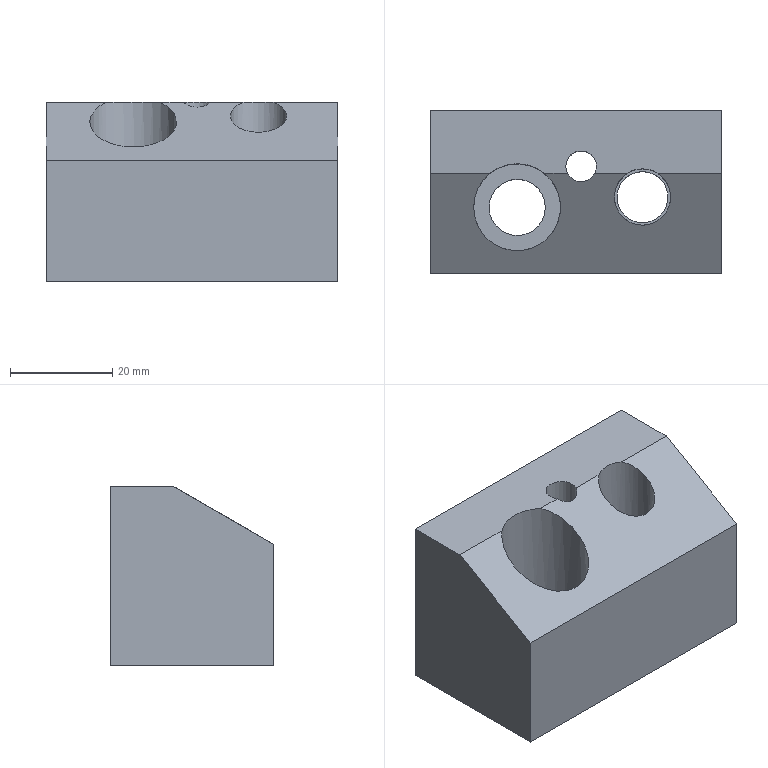Part | STEP file | lll_id4166_x_t | 1 solid | 14 faces | box 57 x 32 x 35 mm | volume 48436 mm3 | plane 9 | cylinder 5 | commonest cylinder face diameters 11 x2 6 x1 10 x1 17 x1
STEP:
#1=CARTESIAN_POINT('',(3855.,-59.75,-35.));
#2=VERTEX_POINT('',#1);
#3=CARTESIAN_POINT('',(3849.5,-59.75,-35.));
#4=DIRECTION('',(0.,0.,1.));
#5=DIRECTION('',(1.,0.,0.));
#6=AXIS2_PLACEMENT_3D('',#3,#4,#5);
#7=CIRCLE('',#6,5.5);
#8=EDGE_CURVE('',#2,#2,#7,.T.);
#9=ORIENTED_EDGE('',*,*,#8,.T.);
#10=EDGE_LOOP('',(#9));
#11=FACE_BOUND('',#10,.T.);
#12=CARTESIAN_POINT('',(3832.5,-40.75,-35.));
#13=VERTEX_POINT('',#12);
#14=CARTESIAN_POINT('',(3832.5,-72.75,-35.));
#15=VERTEX_POINT('',#14);
#16=CARTESIAN_POINT('',(3832.5,-36.5,-35.));
#17=DIRECTION('',(0.,-1.,0.));
#18=VECTOR('',#17,1.);
#19=LINE('',#16,#18);
#20=EDGE_CURVE('',#13,#15,#19,.T.);
#21=ORIENTED_EDGE('',*,*,#20,.F.);
#22=CARTESIAN_POINT('',(3889.5,-40.75,-35.));
#23=VERTEX_POINT('',#22);
#24=CARTESIAN_POINT('',(3854.,-40.75,-35.));
#25=DIRECTION('',(-1.,0.,0.));
#26=VECTOR('',#25,1.);
#27=LINE('',#24,#26);
#28=EDGE_CURVE('',#23,#13,#27,.T.);
#29=ORIENTED_EDGE('',*,*,#28,.F.);
#30=CARTESIAN_POINT('',(3889.5,-72.75,-35.));
#31=VERTEX_POINT('',#30);
#32=CARTESIAN_POINT('',(3889.5,-36.5,-35.));
#33=DIRECTION('',(0.,1.,0.));
#34=VECTOR('',#33,1.);
#35=LINE('',#32,#34);
#36=EDGE_CURVE('',#31,#23,#35,.T.);
#37=ORIENTED_EDGE('',*,*,#36,.F.);
#38=CARTESIAN_POINT('',(3854.,-72.75,-35.));
#39=DIRECTION('',(1.,0.,0.));
#40=VECTOR('',#39,1.);
#41=LINE('',#38,#40);
#42=EDGE_CURVE('',#15,#31,#41,.T.);
#43=ORIENTED_EDGE('',*,*,#42,.F.);
#44=EDGE_LOOP('',(#21,#29,#37,#43));
#45=FACE_BOUND('',#44,.T.);
#46=CARTESIAN_POINT('',(3874.,-62.75,-35.));
#47=VERTEX_POINT('',#46);
#48=CARTESIAN_POINT('',(3874.,-57.75,-35.));
#49=DIRECTION('',(0.,0.,1.));
#50=DIRECTION('',(0.,-1.,0.));
#51=AXIS2_PLACEMENT_3D('',#48,#49,#50);
#52=CIRCLE('',#51,5.);
#53=EDGE_CURVE('',#47,#47,#52,.T.);
#54=ORIENTED_EDGE('',*,*,#53,.T.);
#55=EDGE_LOOP('',(#54));
#56=FACE_BOUND('',#55,.T.);
#57=CARTESIAN_POINT('',(3859.,-51.75,-35.));
#58=VERTEX_POINT('',#57);
#59=CARTESIAN_POINT('',(3862.,-51.75,-35.));
#60=DIRECTION('',(0.,0.,-1.));
#61=DIRECTION('',(-1.,0.,0.));
#62=AXIS2_PLACEMENT_3D('',#59,#60,#61);
#63=CIRCLE('',#62,3.);
#64=EDGE_CURVE('',#58,#58,#63,.T.);
#65=ORIENTED_EDGE('',*,*,#64,.F.);
#66=EDGE_LOOP('',(#65));
#67=FACE_BOUND('',#66,.T.);
#68=CARTESIAN_POINT('',(3854.,-36.5,-35.));
#69=DIRECTION('',(0.,0.,-1.));
#70=DIRECTION('',(0.,-1.,0.));
#71=AXIS2_PLACEMENT_3D('',#68,#69,#70);
#72=PLANE('',#71);
#73=ADVANCED_FACE('',(#11,#45,#56,#67),#72,.T.);
#74=CARTESIAN_POINT('',(3870.966,-53.163,0.));
#75=VERTEX_POINT('',#74);
#76=CARTESIAN_POINT('',(3864.647,-53.163,0.));
#77=VERTEX_POINT('',#76);
#78=CARTESIAN_POINT('',(3854.,-53.163,0.));
#79=DIRECTION('',(-1.,0.,0.));
#80=VECTOR('',#79,1.);
#81=LINE('',#78,#80);
#82=EDGE_CURVE('',#75,#77,#81,.T.);
#83=ORIENTED_EDGE('',*,*,#82,.F.);
#84=CARTESIAN_POINT('',(3877.034,-53.163,0.));
#85=VERTEX_POINT('',#84);
#86=CARTESIAN_POINT('',(3874.,-57.75,0.));
#87=DIRECTION('',(0.,0.,1.));
#88=DIRECTION('',(0.,1.,0.));
#89=AXIS2_PLACEMENT_3D('',#86,#87,#88);
#90=CIRCLE('',#89,5.5);
#91=EDGE_CURVE('',#85,#75,#90,.T.);
#92=ORIENTED_EDGE('',*,*,#91,.F.);
#93=CARTESIAN_POINT('',(3889.5,-53.163,0.));
#94=VERTEX_POINT('',#93);
#95=CARTESIAN_POINT('',(3854.,-53.163,0.));
#96=DIRECTION('',(-1.,0.,0.));
#97=VECTOR('',#96,1.);
#98=LINE('',#95,#97);
#99=EDGE_CURVE('',#94,#85,#98,.T.);
#100=ORIENTED_EDGE('',*,*,#99,.F.);
#101=CARTESIAN_POINT('',(3889.5,-40.75,0.));
#102=VERTEX_POINT('',#101);
#103=CARTESIAN_POINT('',(3889.5,-36.5,0.));
#104=DIRECTION('',(0.,-1.,0.));
#105=VECTOR('',#104,1.);
#106=LINE('',#103,#105);
#107=EDGE_CURVE('',#102,#94,#106,.T.);
#108=ORIENTED_EDGE('',*,*,#107,.F.);
#109=CARTESIAN_POINT('',(3832.5,-40.75,0.));
#110=VERTEX_POINT('',#109);
#111=CARTESIAN_POINT('',(3854.,-40.75,0.));
#112=DIRECTION('',(1.,0.,0.));
#113=VECTOR('',#112,1.);
#114=LINE('',#111,#113);
#115=EDGE_CURVE('',#110,#102,#114,.T.);
#116=ORIENTED_EDGE('',*,*,#115,.F.);
#117=CARTESIAN_POINT('',(3832.5,-53.163,0.));
#118=VERTEX_POINT('',#117);
#119=CARTESIAN_POINT('',(3832.5,-36.5,0.));
#120=DIRECTION('',(0.,1.,0.));
#121=VECTOR('',#120,1.);
#122=LINE('',#119,#121);
#123=EDGE_CURVE('',#118,#110,#122,.T.);
#124=ORIENTED_EDGE('',*,*,#123,.F.);
#125=CARTESIAN_POINT('',(3844.128,-53.163,0.));
#126=VERTEX_POINT('',#125);
#127=CARTESIAN_POINT('',(3854.,-53.163,0.));
#128=DIRECTION('',(-1.,0.,0.));
#129=VECTOR('',#128,1.);
#130=LINE('',#127,#129);
#131=EDGE_CURVE('',#126,#118,#130,.T.);
#132=ORIENTED_EDGE('',*,*,#131,.F.);
#133=CARTESIAN_POINT('',(3854.872,-53.163,0.));
#134=VERTEX_POINT('',#133);
#135=CARTESIAN_POINT('',(3849.5,-59.75,0.));
#136=DIRECTION('',(0.,0.,1.));
#137=DIRECTION('',(-1.,0.,0.));
#138=AXIS2_PLACEMENT_3D('',#135,#136,#137);
#139=CIRCLE('',#138,8.5);
#140=EDGE_CURVE('',#134,#126,#139,.T.);
#141=ORIENTED_EDGE('',*,*,#140,.F.);
#142=CARTESIAN_POINT('',(3859.354,-53.163,0.));
#143=VERTEX_POINT('',#142);
#144=CARTESIAN_POINT('',(3854.,-53.163,0.));
#145=DIRECTION('',(-1.,0.,0.));
#146=VECTOR('',#145,1.);
#147=LINE('',#144,#146);
#148=EDGE_CURVE('',#143,#134,#147,.T.);
#149=ORIENTED_EDGE('',*,*,#148,.F.);
#150=CARTESIAN_POINT('',(3862.,-51.75,0.));
#151=DIRECTION('',(0.,0.,1.));
#152=DIRECTION('',(1.,0.,0.));
#153=AXIS2_PLACEMENT_3D('',#150,#151,#152);
#154=CIRCLE('',#153,3.);
#155=EDGE_CURVE('',#77,#143,#154,.T.);
#156=ORIENTED_EDGE('',*,*,#155,.F.);
#157=EDGE_LOOP('',(#83,#92,#100,#108,#116,#124,#132,#141,#149,#156));
#158=FACE_OUTER_BOUND('',#157,.T.);
#159=CARTESIAN_POINT('',(3854.,-36.5,0.));
#160=DIRECTION('',(0.,0.,1.));
#161=DIRECTION('',(0.,1.,0.));
#162=AXIS2_PLACEMENT_3D('',#159,#160,#161);
#163=PLANE('',#162);
#164=ADVANCED_FACE('',(#158),#163,.T.);
#165=CARTESIAN_POINT('',(3844.,-59.75,-22.));
#166=VERTEX_POINT('',#165);
#167=CARTESIAN_POINT('',(3849.5,-59.75,-22.));
#168=DIRECTION('',(0.,0.,-1.));
#169=DIRECTION('',(-1.,0.,0.));
#170=AXIS2_PLACEMENT_3D('',#167,#168,#169);
#171=CIRCLE('',#170,5.5);
#172=EDGE_CURVE('',#166,#166,#171,.T.);
#173=ORIENTED_EDGE('',*,*,#172,.F.);
#174=EDGE_LOOP('',(#173));
#175=FACE_BOUND('',#174,.T.);
#176=ORIENTED_EDGE('',*,*,#8,.F.);
#177=EDGE_LOOP('',(#176));
#178=FACE_BOUND('',#177,.T.);
#179=CARTESIAN_POINT('',(3849.5,-59.75,-20.));
#180=DIRECTION('',(0.,0.,-1.));
#181=DIRECTION('',(0.,-1.,0.));
#182=AXIS2_PLACEMENT_3D('',#179,#180,#181);
#183=CYLINDRICAL_SURFACE('',#182,5.5);
#184=ADVANCED_FACE('',(#175,#178),#183,.F.);
#185=CARTESIAN_POINT('',(3874.,-52.75,-15.));
#186=VERTEX_POINT('',#185);
#187=CARTESIAN_POINT('',(3874.,-57.75,-15.));
#188=DIRECTION('',(0.,0.,1.));
#189=DIRECTION('',(0.,1.,0.));
#190=AXIS2_PLACEMENT_3D('',#187,#188,#189);
#191=CIRCLE('',#190,5.);
#192=EDGE_CURVE('',#186,#186,#191,.T.);
#193=ORIENTED_EDGE('',*,*,#192,.T.);
#194=EDGE_LOOP('',(#193));
#195=FACE_BOUND('',#194,.T.);
#196=ORIENTED_EDGE('',*,*,#53,.F.);
#197=EDGE_LOOP('',(#196));
#198=FACE_BOUND('',#197,.T.);
#199=CARTESIAN_POINT('',(3874.,-57.75,-20.));
#200=DIRECTION('',(0.,0.,-1.));
#201=DIRECTION('',(0.,1.,0.));
#202=AXIS2_PLACEMENT_3D('',#199,#200,#201);
#203=CYLINDRICAL_SURFACE('',#202,5.);
#204=ADVANCED_FACE('',(#195,#198),#203,.F.);
#205=CARTESIAN_POINT('',(3874.,-52.25,-15.));
#206=VERTEX_POINT('',#205);
#207=CARTESIAN_POINT('',(3874.,-57.75,-15.));
#208=DIRECTION('',(0.,0.,1.));
#209=DIRECTION('',(0.,1.,0.));
#210=AXIS2_PLACEMENT_3D('',#207,#208,#209);
#211=CIRCLE('',#210,5.5);
#212=EDGE_CURVE('',#206,#206,#211,.T.);
#213=ORIENTED_EDGE('',*,*,#212,.T.);
#214=EDGE_LOOP('',(#213));
#215=FACE_BOUND('',#214,.T.);
#216=ORIENTED_EDGE('',*,*,#192,.F.);
#217=EDGE_LOOP('',(#216));
#218=FACE_BOUND('',#217,.T.);
#219=CARTESIAN_POINT('',(3874.,-57.75,-15.));
#220=DIRECTION('',(0.,0.,-1.));
#221=DIRECTION('',(0.,1.,0.));
#222=AXIS2_PLACEMENT_3D('',#219,#220,#221);
#223=PLANE('',#222);
#224=ADVANCED_FACE('',(#215,#218),#223,.F.);
#225=ORIENTED_EDGE('',*,*,#28,.T.);
#226=CARTESIAN_POINT('',(3832.5,-40.75,-65.));
#227=DIRECTION('',(0.,0.,-1.));
#228=VECTOR('',#227,1.);
#229=LINE('',#226,#228);
#230=EDGE_CURVE('',#110,#13,#229,.T.);
#231=ORIENTED_EDGE('',*,*,#230,.F.);
#232=ORIENTED_EDGE('',*,*,#115,.T.);
#233=CARTESIAN_POINT('',(3889.5,-40.75,-65.));
#234=DIRECTION('',(0.,0.,-1.));
#235=VECTOR('',#234,1.);
#236=LINE('',#233,#235);
#237=EDGE_CURVE('',#102,#23,#236,.T.);
#238=ORIENTED_EDGE('',*,*,#237,.T.);
#239=EDGE_LOOP('',(#225,#231,#232,#238));
#240=FACE_OUTER_BOUND('',#239,.T.);
#241=CARTESIAN_POINT('',(3854.,-40.75,-65.));
#242=DIRECTION('',(0.,1.,0.));
#243=DIRECTION('',(0.,0.,-1.));
#244=AXIS2_PLACEMENT_3D('',#241,#242,#243);
#245=PLANE('',#244);
#246=ADVANCED_FACE('',(#240),#245,.T.);
#247=CARTESIAN_POINT('',(3889.5,-72.75,-11.309));
#248=VERTEX_POINT('',#247);
#249=CARTESIAN_POINT('',(3889.5,-72.75,-65.));
#250=DIRECTION('',(0.,0.,-1.));
#251=VECTOR('',#250,1.);
#252=LINE('',#249,#251);
#253=EDGE_CURVE('',#248,#31,#252,.T.);
#254=ORIENTED_EDGE('',*,*,#253,.T.);
#255=ORIENTED_EDGE('',*,*,#36,.T.);
#256=ORIENTED_EDGE('',*,*,#237,.F.);
#257=ORIENTED_EDGE('',*,*,#107,.T.);
#258=CARTESIAN_POINT('',(3889.5,-68.812,-9.035));
#259=DIRECTION('',(0.,0.866,0.5));
#260=VECTOR('',#259,1.);
#261=LINE('',#258,#260);
#262=EDGE_CURVE('',#248,#94,#261,.T.);
#263=ORIENTED_EDGE('',*,*,#262,.F.);
#264=EDGE_LOOP('',(#254,#255,#256,#257,#263));
#265=FACE_OUTER_BOUND('',#264,.T.);
#266=CARTESIAN_POINT('',(3889.5,-36.5,-65.));
#267=DIRECTION('',(1.,0.,0.));
#268=DIRECTION('',(0.,0.,-1.));
#269=AXIS2_PLACEMENT_3D('',#266,#267,#268);
#270=PLANE('',#269);
#271=ADVANCED_FACE('',(#265),#270,.T.);
#272=CARTESIAN_POINT('',(3832.5,-72.75,-11.309));
#273=VERTEX_POINT('',#272);
#274=CARTESIAN_POINT('',(3832.5,-72.75,-65.));
#275=DIRECTION('',(0.,0.,-1.));
#276=VECTOR('',#275,1.);
#277=LINE('',#274,#276);
#278=EDGE_CURVE('',#273,#15,#277,.T.);
#279=ORIENTED_EDGE('',*,*,#278,.T.);
#280=ORIENTED_EDGE('',*,*,#42,.T.);
#281=ORIENTED_EDGE('',*,*,#253,.F.);
#282=CARTESIAN_POINT('',(3854.,-72.75,-11.309));
#283=DIRECTION('',(1.,0.,0.));
#284=VECTOR('',#283,1.);
#285=LINE('',#282,#284);
#286=EDGE_CURVE('',#273,#248,#285,.T.);
#287=ORIENTED_EDGE('',*,*,#286,.F.);
#288=EDGE_LOOP('',(#279,#280,#281,#287));
#289=FACE_OUTER_BOUND('',#288,.T.);
#290=CARTESIAN_POINT('',(3854.,-72.75,-65.));
#291=DIRECTION('',(0.,-1.,0.));
#292=DIRECTION('',(0.,0.,1.));
#293=AXIS2_PLACEMENT_3D('',#290,#291,#292);
#294=PLANE('',#293);
#295=ADVANCED_FACE('',(#289),#294,.T.);
#296=ORIENTED_EDGE('',*,*,#123,.T.);
#297=ORIENTED_EDGE('',*,*,#230,.T.);
#298=ORIENTED_EDGE('',*,*,#20,.T.);
#299=ORIENTED_EDGE('',*,*,#278,.F.);
#300=CARTESIAN_POINT('',(3832.5,-68.812,-9.035));
#301=DIRECTION('',(0.,-0.866,-0.5));
#302=VECTOR('',#301,1.);
#303=LINE('',#300,#302);
#304=EDGE_CURVE('',#118,#273,#303,.T.);
#305=ORIENTED_EDGE('',*,*,#304,.F.);
#306=EDGE_LOOP('',(#296,#297,#298,#299,#305));
#307=FACE_OUTER_BOUND('',#306,.T.);
#308=CARTESIAN_POINT('',(3832.5,-36.5,-65.));
#309=DIRECTION('',(-1.,0.,0.));
#310=DIRECTION('',(0.,0.,1.));
#311=AXIS2_PLACEMENT_3D('',#308,#309,#310);
#312=PLANE('',#311);
#313=ADVANCED_FACE('',(#307),#312,.T.);
#314=CARTESIAN_POINT('',(3874.,-57.75,-2.648));
#315=DIRECTION('',(0.,-0.5,0.866));
#316=DIRECTION('',(0.,-0.866,-0.5));
#317=AXIS2_PLACEMENT_3D('',#314,#315,#316);
#318=ELLIPSE('',#317,6.351,5.5);
#319=EDGE_CURVE('',#75,#85,#318,.T.);
#320=ORIENTED_EDGE('',*,*,#319,.T.);
#321=ORIENTED_EDGE('',*,*,#91,.T.);
#322=EDGE_LOOP('',(#320,#321));
#323=FACE_BOUND('',#322,.T.);
#324=ORIENTED_EDGE('',*,*,#212,.F.);
#325=EDGE_LOOP('',(#324));
#326=FACE_BOUND('',#325,.T.);
#327=CARTESIAN_POINT('',(3874.,-57.75,0.));
#328=DIRECTION('',(0.,0.,-1.));
#329=DIRECTION('',(0.,1.,0.));
#330=AXIS2_PLACEMENT_3D('',#327,#328,#329);
#331=CYLINDRICAL_SURFACE('',#330,5.5);
#332=ADVANCED_FACE('',(#323,#326),#331,.F.);
#333=ORIENTED_EDGE('',*,*,#172,.T.);
#334=EDGE_LOOP('',(#333));
#335=FACE_BOUND('',#334,.T.);
#336=CARTESIAN_POINT('',(3841.,-59.75,-22.));
#337=VERTEX_POINT('',#336);
#338=CARTESIAN_POINT('',(3849.5,-59.75,-22.));
#339=DIRECTION('',(0.,0.,1.));
#340=DIRECTION('',(-1.,0.,0.));
#341=AXIS2_PLACEMENT_3D('',#338,#339,#340);
#342=CIRCLE('',#341,8.5);
#343=EDGE_CURVE('',#337,#337,#342,.T.);
#344=ORIENTED_EDGE('',*,*,#343,.T.);
#345=EDGE_LOOP('',(#344));
#346=FACE_BOUND('',#345,.T.);
#347=CARTESIAN_POINT('',(3849.5,-59.75,-22.));
#348=DIRECTION('',(0.,0.,-1.));
#349=DIRECTION('',(0.,-1.,0.));
#350=AXIS2_PLACEMENT_3D('',#347,#348,#349);
#351=PLANE('',#350);
#352=ADVANCED_FACE('',(#335,#346),#351,.F.);
#353=ORIENTED_EDGE('',*,*,#343,.F.);
#354=EDGE_LOOP('',(#353));
#355=FACE_BOUND('',#354,.T.);
#356=ORIENTED_EDGE('',*,*,#140,.T.);
#357=CARTESIAN_POINT('',(3849.5,-59.75,-3.803));
#358=DIRECTION('',(0.,0.5,-0.866));
#359=DIRECTION('',(0.,0.866,0.5));
#360=AXIS2_PLACEMENT_3D('',#357,#358,#359);
#361=ELLIPSE('',#360,9.815,8.5);
#362=EDGE_CURVE('',#134,#126,#361,.T.);
#363=ORIENTED_EDGE('',*,*,#362,.F.);
#364=EDGE_LOOP('',(#356,#363));
#365=FACE_BOUND('',#364,.T.);
#366=CARTESIAN_POINT('',(3849.5,-59.75,-20.));
#367=DIRECTION('',(0.,0.,1.));
#368=DIRECTION('',(0.,1.,0.));
#369=AXIS2_PLACEMENT_3D('',#366,#367,#368);
#370=CYLINDRICAL_SURFACE('',#369,8.5);
#371=ADVANCED_FACE('',(#355,#365),#370,.F.);
#372=ORIENTED_EDGE('',*,*,#155,.T.);
#373=CARTESIAN_POINT('',(3862.,-51.75,0.8156));
#374=DIRECTION('',(0.,0.5,-0.866));
#375=DIRECTION('',(0.,-0.866,-0.5));
#376=AXIS2_PLACEMENT_3D('',#373,#374,#375);
#377=ELLIPSE('',#376,3.464,3.);
#378=EDGE_CURVE('',#77,#143,#377,.T.);
#379=ORIENTED_EDGE('',*,*,#378,.F.);
#380=EDGE_LOOP('',(#372,#379));
#381=FACE_BOUND('',#380,.T.);
#382=ORIENTED_EDGE('',*,*,#64,.T.);
#383=EDGE_LOOP('',(#382));
#384=FACE_BOUND('',#383,.T.);
#385=CARTESIAN_POINT('',(3862.,-51.75,15.));
#386=DIRECTION('',(0.,0.,-1.));
#387=DIRECTION('',(1.,0.,0.));
#388=AXIS2_PLACEMENT_3D('',#385,#386,#387);
#389=CYLINDRICAL_SURFACE('',#388,3.);
#390=ADVANCED_FACE('',(#381,#384),#389,.F.);
#391=ORIENTED_EDGE('',*,*,#378,.T.);
#392=ORIENTED_EDGE('',*,*,#148,.T.);
#393=ORIENTED_EDGE('',*,*,#362,.T.);
#394=ORIENTED_EDGE('',*,*,#131,.T.);
#395=ORIENTED_EDGE('',*,*,#304,.T.);
#396=ORIENTED_EDGE('',*,*,#286,.T.);
#397=ORIENTED_EDGE('',*,*,#262,.T.);
#398=ORIENTED_EDGE('',*,*,#99,.T.);
#399=ORIENTED_EDGE('',*,*,#319,.F.);
#400=ORIENTED_EDGE('',*,*,#82,.T.);
#401=EDGE_LOOP('',(#391,#392,#393,#394,#395,#396,#397,#398,#399,#400));
#402=FACE_OUTER_BOUND('',#401,.T.);
#403=CARTESIAN_POINT('',(3816.5,-93.,-23.));
#404=DIRECTION('',(0.,0.5,-0.866));
#405=DIRECTION('',(1.,0.,0.));
#406=AXIS2_PLACEMENT_3D('',#403,#404,#405);
#407=PLANE('',#406);
#408=ADVANCED_FACE('',(#402),#407,.F.);
#409=CLOSED_SHELL('',(#73,#164,#184,#204,#224,#246,#271,#295,#313,#332,#352,#371,#390,#408));
#410=MANIFOLD_SOLID_BREP('',#409);
#411=(LENGTH_UNIT()NAMED_UNIT(*)SI_UNIT(.MILLI.,.METRE.));
#412=UNCERTAINTY_MEASURE_WITH_UNIT(LENGTH_MEASURE(0.00002),#411,'','');
#413=(NAMED_UNIT(*)PLANE_ANGLE_UNIT()SI_UNIT($,.RADIAN.));
#414=PLANE_ANGLE_MEASURE_WITH_UNIT(PLANE_ANGLE_MEASURE(0.01745),#413);
#415=DIMENSIONAL_EXPONENTS(0.,0.,0.,0.,0.,0.,0.);
#416=(CONVERSION_BASED_UNIT('DEGREE',#414)NAMED_UNIT(#415)PLANE_ANGLE_UNIT());
#417=(NAMED_UNIT(*)SI_UNIT($,.STERADIAN.)SOLID_ANGLE_UNIT());
#418=(GEOMETRIC_REPRESENTATION_CONTEXT(3)GLOBAL_UNCERTAINTY_ASSIGNED_CONTEXT((#412))GLOBAL_UNIT_ASSIGNED_CONTEXT((#411,#416,#417))REPRESENTATION_CONTEXT('',''));
#419=ADVANCED_BREP_SHAPE_REPRESENTATION('',(#410),#418);